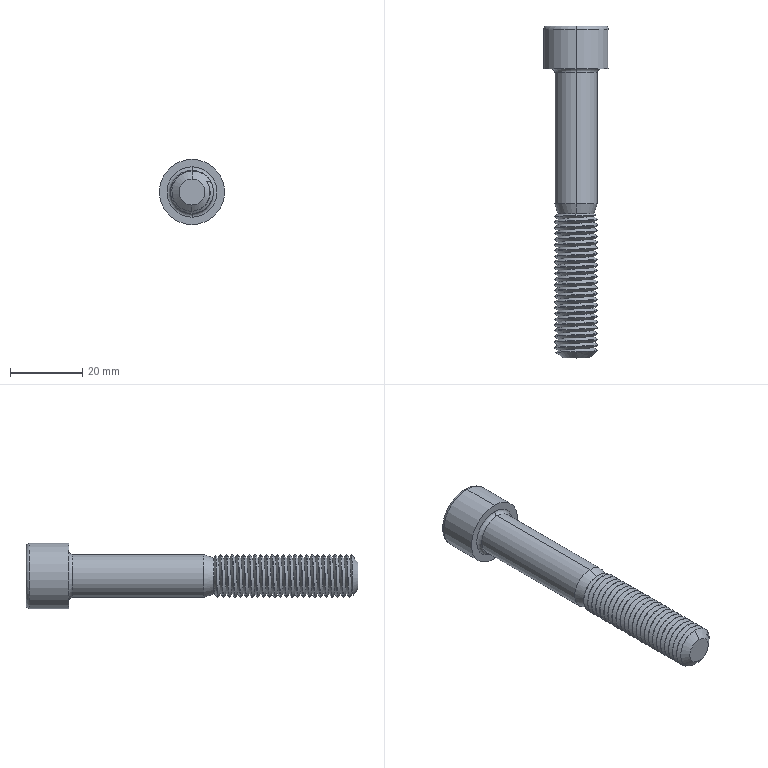Part | STEP file | Parafuso M12 - 80mm | 1 solid | 79 faces | box 18.1 x 91.8 x 18.1 mm | volume 10767 mm3 | cylinder 52 | plane 10 | cone 9 | torus 6 | spline 2 | commonest cylinder face diameters 11.9 x50 18.1 x2